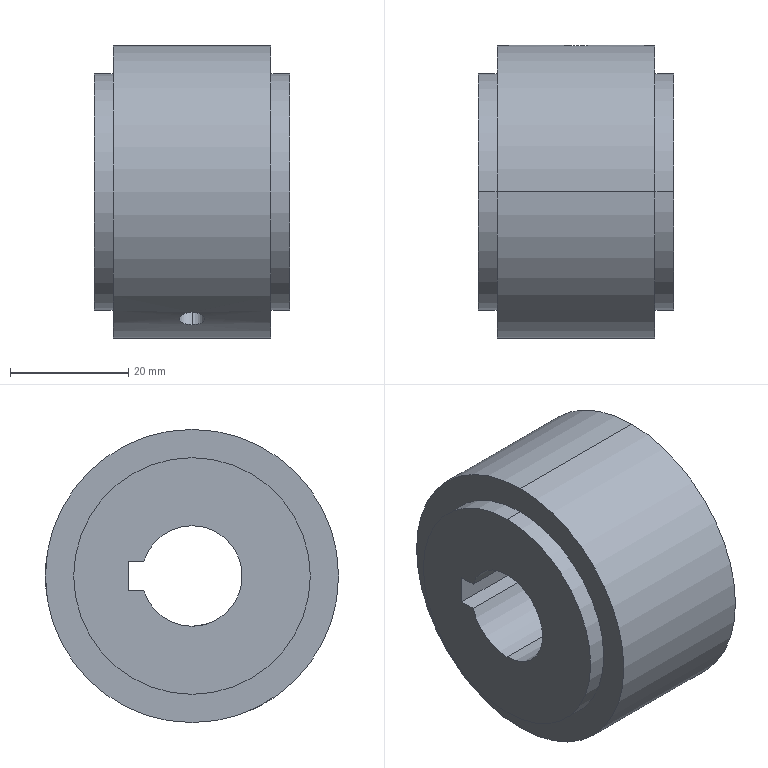Part | STEP file | 0245_006_GPM20YU8250-A-N17-NFC | 1 solid | 20 faces | box 33 x 49.56 x 49.56 mm | volume 51114 mm3 | cylinder 13 | plane 7 | commonest cylinder face diameters 4.2 x4 40 x4 17 x3 49.56 x2